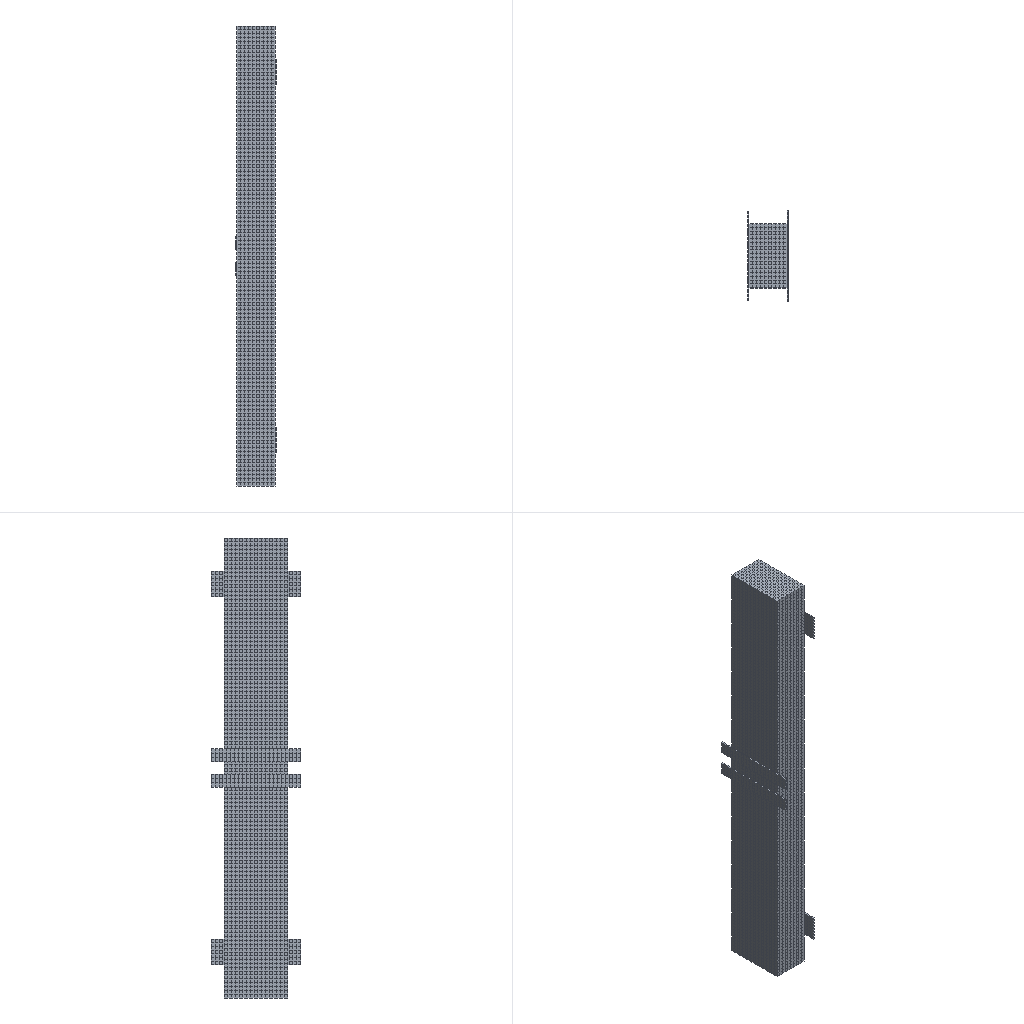Simulation study | abaqus
Set-up summary:
category,name,step,type,value,unit,region
solver,abaqus
solver,version,,,Abaqus/Explicit 2020
units,not stated in the deck,,not stated
analysis,deck,,transient,transient
load_step,Step-1,Step-1,transient,nlgeom=True
contact,interactions,,,general=1 pairs=0 ties=0
load_step,requested,,,1
mesh,nodes,,,26658
mesh,elements,,,22464
element_type,T3D2,,truss,1604
element_type,C3D8R,,solid,20860
load,load commands in deck,,count,1
bc,support commands in deck,,count,6
material,CON,,in results
material,STEEL-10,,in results
material,STEEL-8,,in results
material,STEEL8-25,,in results
check,setup vs results,,match,"per instance, exact: element labels, types and connectivity; labels of the nodes the elements use; coordinates of those nodes at SINGLE_PRECISION in 6 of 6 instance(s)"
Abaqus input file, long lists of numbers shortened:
*Heading
** Job name: Job-2 Model name: Model-1-s
** Generated by: Abaqus/CAE 2020
*Preprint, echo=NO, model=NO, history=NO, contact=NO
**
** PARTS
**
*Part, name=con
*Node
      1,           0.,        -250.,        1800.
      2,           0.,  -235.294,        1800.
** (23956 more lines like these left out)
*Element, type=C3D8R
    1,  2179,  2180,  2198,  2197,     1,     2,    20,    19
    2,  2180,  2181,  2199,  2198,     2,     3,    21,    20
** (20398 more lines like these left out)
*Nset, nset=Set-1, generate
     1,  23958,      1
*Elset, elset=Set-1, generate
     1,  20400,      1
** Section: con
*Solid Section, elset=Set-1, material=con
,
*End Part
**
*Part, name=jin-fianl
*Node
      1,          25.,        -225.,          25.
      2,          25.,         -25.,          25.
** (1546 more lines like these left out)
*Element, type=T3D2
 1,  2, 61
 2, 61, 62
** (1602 more lines like these left out)
*Nset, nset=Set-1, generate
    1,  1548,     1
*Elset, elset=Set-1, generate
    1,  1604,     1
** Section: j10
*Solid Section, elset=Set-1, material=steel-10
78.5,
*End Part
**
*Part, name=rig
*Node
      1,         -50.,        -100.,           5.
      2,         -50.,  -85.714,           5.
** (382 more lines like these left out)
*Element, type=C3D8R
  1,  17,  18,  26,  25,   1,   2,  10,   9
  2,  18,  19,  27,  26,   2,   3,  11,  10
** (159 more lines like these left out)
*Nset, nset=Set-1, generate
   1,  384,    1
*Elset, elset=Set-1, generate
   1,  161,    1
** Section: s
*Solid Section, elset=Set-1, material=steel-8
,
*End Part
**
*Part, name=rig-z
*Node
      1,           0.,      -273.75,           5.
      2,           0.,  -258.533,           5.
** (190 more lines like these left out)
*Element, type=C3D8R
 1,  49,  50,  74,  73,   1,   2,  26,  25
 2,  50,  51,  75,  74,   2,   3,  27,  26
** (67 more lines like these left out)
*Nset, nset=Set-1, generate
   1,  192,    1
*Elset, elset=Set-1, generate
  1,  69,   1
** Section: s
*Solid Section, elset=Set-1, material=steel-8
,
*End Part
**
**
** ASSEMBLY
**
*Assembly, name=Assembly
**
*Instance, name=con-1, part=con
*End Instance
**
*Instance, name=rig-1, part=rig
        155.,           0.,         230.
        155.,           0.,         230., 155.577, -0.5774, 229.423,         120.
*End Instance
**
*Instance, name=rig-1-lin-2-1, part=rig
        155.,           0.,        1670.
        155.,           0.,        1670., 155.577, -0.5774, 1669.423,         120.
*End Instance
**
*Instance, name=jin-fianl-1, part=jin-fianl
*End Instance
**
*Instance, name=rig-z-2, part=rig-z
         -5.,       -26.25,         975.
         -5.,       -26.25,         975.,          -5., -25.25,         975., 90.
*End Instance
**
*Instance, name=rig-z-2-lin-2-1, part=rig-z
         -5.,       -26.25,         875.
         -5.,       -26.25,         875.,          -5., -25.25,         875., 90.
*End Instance
**
*Node
      1,           0.,        -125.,         900.
*Node
      2,         150.,        -125.,         900.
*Nset, nset=Set-5, instance=con-1, generate
     1,  23958,      1
*Nset, nset=Set-5, instance=jin-fianl-1, generate
    1,  1548,     1
*Elset, elset=Set-5, instance=con-1, generate
     1,  20400,      1
*Elset, elset=Set-5, instance=jin-fianl-1, generate
    1,  1604,     1
*Nset, nset=Set-6
 2,
*Nset, nset=Set-7, instance=con-1, generate
     1,  23958,      1
*Nset, nset=Set-7, instance=jin-fianl-1, generate
    1,  1548,     1
*Elset, elset=Set-7, instance=con-1, generate
     1,  20400,      1
*Elset, elset=Set-7, instance=jin-fianl-1, generate
    1,  1604,     1
*Nset, nset=Set-8
 1,
*Nset, nset=Set-9
 1,
*Nset, nset=b_Set-1, instance=rig-1, generate
   1,  384,    1
*Nset, nset=b_Set-1, instance=rig-1-lin-2-1, generate
   1,  384,    1
*Elset, elset=b_Set-1, instance=rig-1, generate
   1,  161,    1
*Elset, elset=b_Set-1, instance=rig-1-lin-2-1, generate
   1,  161,    1
*Nset, nset=b_Set-9, instance=rig-1, generate
   1,  384,    1
*Nset, nset=b_Set-9, instance=rig-1-lin-2-1, generate
   1,  384,    1
*Elset, elset=b_Set-9, instance=rig-1, generate
   1,  161,    1
*Elset, elset=b_Set-9, instance=rig-1-lin-2-1, generate
   1,  161,    1
*Nset, nset=b_Set-13, instance=rig-z-2, generate
   1,  192,    1
*Nset, nset=b_Set-13, instance=rig-z-2-lin-2-1, generate
   1,  192,    1
*Elset, elset=b_Set-13, instance=rig-z-2, generate
  1,  69,   1
*Elset, elset=b_Set-13, instance=rig-z-2-lin-2-1, generate
  1,  69,   1
*Nset, nset=m_Set-3, instance=jin-fianl-1, generate
    1,  1548,     1
*Elset, elset=m_Set-3, instance=jin-fianl-1, generate
    1,  1604,     1
*Nset, nset=s_Set-3, instance=con-1, generate
     1,  23958,      1
*Elset, elset=s_Set-3, instance=con-1, generate
     1,  20400,      1
*Nset, nset=_PickedSet79, internal
 2,
*Nset, nset=_PickedSet81, internal
 1,
*Elset, elset=_Surf-1_S1, internal, instance=con-1, generate
 18361,  20400,      1
*Elset, elset=_Surf-1_S6, internal, instance=con-1, generate
     1,  20384,     17
*Elset, elset=_Surf-1_S4, internal, instance=con-1, generate
    17,  20400,     17
*Surface, type=ELEMENT, name=Surf-1
_Surf-1_S1, S1
_Surf-1_S6, S6
_Surf-1_S4, S4
*Elset, elset=_Surf-2_S1, internal, instance=con-1, generate
 18361,  20400,      1
*Elset, elset=_Surf-2_S6, internal, instance=con-1, generate
     1,  20384,     17
*Elset, elset=_Surf-2_S4, internal, instance=con-1, generate
    17,  20400,     17
*Surface, type=ELEMENT, name=Surf-2
_Surf-2_S1, S1
_Surf-2_S6, S6
_Surf-2_S4, S4
*Elset, elset=_m_Surf-5_S3, internal, instance=rig-1, generate
   1,  161,    1
*Elset, elset=_m_Surf-5_S3, internal, instance=rig-1-lin-2-1, generate
   1,  161,    1
*Surface, type=ELEMENT, name=m_Surf-5
_m_Surf-5_S3, S3
*Elset, elset=_m_Surf-9_S3, internal, instance=rig-1, generate
   1,  161,    1
*Elset, elset=_m_Surf-9_S3, internal, instance=rig-1-lin-2-1, generate
   1,  161,    1
*Surface, type=ELEMENT, name=m_Surf-9
_m_Surf-9_S3, S3
*Elset, elset=_m_Surf-13_S3, internal, instance=rig-1, generate
   1,  161,    1
*Elset, elset=_m_Surf-13_S3, internal, instance=rig-1-lin-2-1, generate
   1,  161,    1
*Surface, type=ELEMENT, name=m_Surf-13
_m_Surf-13_S3, S3
*Elset, elset=_m_Surf-17_S1, internal, instance=con-1, generate
 18361,  20400,      1
*Surface, type=ELEMENT, name=m_Surf-17
_m_Surf-17_S1, S1
*Elset, elset=_s_Surf-3_S2, internal, instance=con-1, generate
    1,  2040,     1
*Surface, type=ELEMENT, name=s_Surf-3
_s_Surf-3_S2, S2
*Elset, elset=_s_Surf-5_S1, internal, instance=con-1, generate
 18361,  20400,      1
*Surface, type=ELEMENT, name=s_Surf-5
_s_Surf-5_S1, S1
*Elset, elset=_s_Surf-7_S2, internal, instance=con-1, generate
    1,  2040,     1
*Surface, type=ELEMENT, name=s_Surf-7
_s_Surf-7_S2, S2
*Elset, elset=_s_Surf-9_S1, internal, instance=con-1, generate
 18361,  20400,      1
*Surface, type=ELEMENT, name=s_Surf-9
_s_Surf-9_S1, S1
*Elset, elset=_s_Surf-11_S2, internal, instance=con-1, generate
    1,  2040,     1
*Surface, type=ELEMENT, name=s_Surf-11
_s_Surf-11_S2, S2
*Elset, elset=_s_Surf-13_S1, internal, instance=con-1, generate
 18361,  20400,      1
*Surface, type=ELEMENT, name=s_Surf-13
_s_Surf-13_S1, S1
*Elset, elset=_s_Surf-15_S2, internal, instance=con-1, generate
    1,  2040,     1
*Surface, type=ELEMENT, name=s_Surf-15
_s_Surf-15_S2, S2
*Elset, elset=_s_Surf-17_S3, internal, instance=rig-1, generate
   1,  161,    1
*Elset, elset=_s_Surf-17_S3, internal, instance=rig-1-lin-2-1, generate
   1,  161,    1
*Surface, type=ELEMENT, name=s_Surf-17
_s_Surf-17_S3, S3
** Constraint: Constraint-2
*Embedded Element, host elset=s_Set-3
m_Set-3
** Constraint: Constraint-3
*Rigid Body, ref node=_PickedSet79, elset=b_Set-9
** Constraint: Constraint-4
*Rigid Body, ref node=_PickedSet81, elset=b_Set-13
*End Assembly
*Amplitude, name=Amp-1
             0.,              0.,           1000.,            120.,           2000.,            300.,           3000.,            500.
          4000.,            670.,           5000.,            850.,           6000.,           1100.,           7000.,           1200.
          8000.,           1350.,           9000.,           1500.,          10000.,           1400.,          11000.,           1450.
*Amplitude, name=Amp-2
             0.,              0.,             0.1,              1.
**
** MATERIALS
**
*Material, name=con
*Conductivity
 1.28,
*Density
 2.5e-09,
*Elastic
32500., 0.2
*Expansion
 1e-05,
*Specific Heat
 8.4e+08,
*Concrete Damaged Plasticity
30.,   0.1,  1.16, 0.667,  0.01
*Concrete Compression Hardening
 31.839,          0.
  35.238, 0.0001688
  37.656, 0.0002734
 39.058, 0.0004092
    39.5, 0.0005746
 38.815, 0.0007747
 37.101,  0.001006
  34.823,  0.001256
 32.332,  0.001511
 29.849,  0.001767
 27.497,  0.002018
 25.334,   0.002263
 23.376,  0.002503
 21.619,  0.002736
 20.051,  0.002963
 18.651,  0.003185
 17.402,  0.003403
 16.285,  0.003616
 15.284,  0.003826
 14.385,   0.004032
 13.573,  0.004236
 12.839,  0.004438
 12.173,  0.004637
 11.567,   0.004835
  11.013,  0.005031
*Concrete Tension Stiffening
  2.09,       0.
   2.4, 8.74e-06
  2.67, 1.23e-05
  2.86, 1.81e-05
  2.94, 2.75e-05
   2.8, 4.37e-05
  2.55, 6.31e-05
   2.3, 8.27e-05
  2.07, 0.000102
  1.86,  0.00012
  1.69, 0.000137
  1.55, 0.000153
  1.42, 0.000169
  1.31, 0.000184
  1.22, 0.000198
  1.14, 0.000213
  1.07, 0.000227
  1.01,  0.00024
 0.956, 0.000254
 0.908, 0.000267
 0.864,  0.00028
 0.825, 0.000293
 0.789, 0.000306
 0.757, 0.000319
 0.727, 0.000332
*Concrete Compression Damage
        0.,          0.
 0.06977, 0.0001688
  0.1005, 0.0002734
  0.1363, 0.0004092
  0.176, 0.0005746
  0.2212, 0.0007747
  0.271,  0.001006
  0.3214,  0.001256
  0.3699,  0.001511
  0.4151,  0.001767
  0.4565,  0.002018
  0.4939,   0.002263
  0.5275,  0.002503
   0.5577,  0.002736
  0.5849,  0.002963
   0.6093,  0.003185
  0.6313,  0.003403
  0.6511,  0.003616
  0.6691,  0.003826
  0.6855,   0.004032
  0.7004,  0.004236
  0.7141,  0.004438
  0.7266,  0.004637
  0.7382,   0.004835
  0.7488,  0.005031
  0.7586,  0.005226
  0.7678,  0.005419
  0.7763,  0.005611
  0.7842,  0.005802
  0.7915,  0.005993
  0.7984,  0.006182
  0.8049,  0.006371
  0.811,  0.006559
  0.8167,  0.006747
  0.8221,  0.006933
  0.8627,  0.008781
  0.8884,   0.01061
  0.906,   0.01242
  0.9188,   0.01423
  0.9286,   0.01603
** (21 more lines like these left out)
*Concrete Tension Damage, compression recovery=0.45
     0.,       0.
 0.0544, 8.74e-06
 0.0674, 1.23e-05
 0.0893, 1.81e-05
  0.124, 2.75e-05
  0.186, 4.37e-05
  0.255, 6.31e-05
  0.321, 8.27e-05
   0.38, 0.000102
  0.431,  0.00012
  0.475, 0.000137
  0.513, 0.000153
  0.546, 0.000169
  0.575, 0.000184
  0.601, 0.000198
  0.623, 0.000213
  0.643, 0.000227
  0.661,  0.00024
  0.678, 0.000254
  0.692, 0.000267
  0.706,  0.00028
  0.718, 0.000293
  0.729, 0.000306
  0.739, 0.000319
  0.749, 0.000332
  0.757, 0.000344
  0.765, 0.000357
  0.773, 0.000369
   0.78, 0.000382
  0.787, 0.000394
  0.793, 0.000407
  0.799, 0.000419
  0.804, 0.000431
  0.809, 0.000443
  0.814, 0.000456
  0.851, 0.000577
  0.875, 0.000697
  0.892, 0.000816
  0.905, 0.000935
  0.915,  0.00105
** (31 more lines like these left out)
*Material, name=steel-8
*Conductivity
50.,
*Density
 7.8e-09,
*Elastic
205000., 0.3
*Expansion
 1.5e-05,
*Plastic
469.,0.
*Specific Heat
 4.6e+08,
*Material, name=steel-10
*Conductivity
50.,
*Density
 7.8e-09,
*Elastic
205000., 0.3
*Expansion
 1.5e-05,
*Plastic
468.,0.
*Specific Heat
 4.6e+08,
*Material, name=steel8-25
*Conductivity
50.,
*Density
 7.8e-09,
*Elastic
205000., 0.3
*Expansion
 1.5e-05,
*Plastic
433.,0.
*Specific Heat
 4.6e+08,
**
** INTERACTION PROPERTIES
**
*Surface Interaction, name=IntProp-1
*Friction
 0.1,
*Surface Behavior, pressure-overclosure=HARD
**
** PHYSICAL CONSTANTS
**
*Physical Constants, absolute zero=-273., stefan boltzmann=5.67e-08
**
** PREDEFINED FIELDS
**
** Name: Predefined Field-1   Type: Temperature
*Initial Conditions, type=TEMPERATURE
Set-5, 20.
** ----------------------------------------------------------------
**
** STEP: Step-1
**
*Step, name=Step-1, nlgeom=YES
*Dynamic, Explicit
, 0.1
*Bulk Viscosity
0.06, 1.2
**
** BOUNDARY CONDITIONS
**
** Name: BC-1 Type: 对称/反对称/完全固定
*Boundary
Set-6, ENCASTRE
** Name: BC-2 Type: 位移/转角
*Boundary
Set-8, 2, 2
Set-8, 3, 3
Set-8, 4, 4
Set-8, 5, 5
Set-8, 6, 6
**
** LOADS
**
** Name: Load-1   Type: Concentrated force
*Cload, amplitude=Amp-2
Set-9, 1, 24000.
**
** PREDEFINED FIELDS
**
** Name: Predefined Field-2   Type: Temperature
*Temperature, file=D:\LiangTEMPstress\model\Job-1.odb, bstep=1, binc=1, estep=1, einc=50
**
** INTERACTIONS
**
** Interaction: Int-3
*Contact, op=NEW
*Contact Inclusions, ALL EXTERIOR
*Contact Property Assignment
 ,  , IntProp-1
**
** OUTPUT REQUESTS
**
*Restart, write, number interval=1, time marks=NO
**
** FIELD OUTPUT: F-Output-1
**
*Output, field
*Node Output
CF, RF, RM, RT, U, V
*Element Output, directions=YES
CTSHR, DAMAGEC, DAMAGET, DMICRT, E, LE, MISES, MISESMAX, MISESONLY, NE, PE, PEEQ, PEEQMAX, PEEQT, PEMAG, PRESSONLY
S, SDEG, SE, SEQUT, SF, SSAVG, STATUS, TEMP, TRIAX, TSHR, VEEQ, YIELDPOT
*Element Output, rebar, directions=YES
CTSHR, DAMAGEC, DAMAGET, DMICRT, E, LE, MISES, MISESMAX, MISESONLY, NE, PE, PEEQ, PEEQMAX, PEEQT, PEMAG, PRESSONLY
S, SDEG, SE, SEQUT, SF, SSAVG, STATUS, TEMP, TRIAX, TSHR, VEEQ, YIELDPOT
*Contact Output
CDISP, CFORCE, CSTRESS, PPRESS
**
** HISTORY OUTPUT: H-Output-1
**
*Output, history, time interval=1e-05
*Node Output, nset=Set-8
RF1, U1
*End Step
Results summary:
result,step,Step-1,completed,increments=58619 time=0.1/0.1
result,analysis,,,transient
result,last_loadstep,,,1
result,analysis steps,,count,1
result,primary field,,,U
result,reaction total,,FX,-24915.336,model units
result,reaction total,,FY,-469.2,model units
result,reaction total,,FZ,-69.381,model units